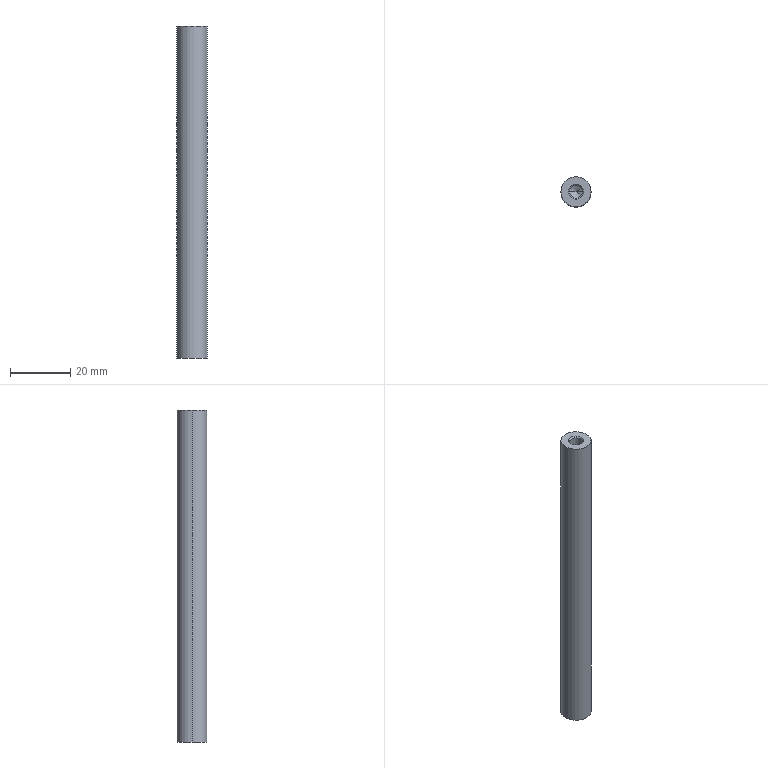Part | SolidWorks | features 3DProfileFeature 1, Extrusion 1, HoleWzd 1, MirrorPattern 1 | 1 solid | 16 faces | box 10 x 10 x 110 mm | volume 8282 mm3 | cone 8 | cylinder 6 | plane 2 | commonest cylinder face diameters 4.2 x4 10 x2
STEP:
#1=CARTESIAN_POINT('',(2.1,0.,-54.575));
#2=VERTEX_POINT('',#1);
#3=CARTESIAN_POINT('',(-2.1,0.,-54.575));
#4=VERTEX_POINT('',#3);
#5=CARTESIAN_POINT('',(0.,0.,-54.575));
#6=DIRECTION('',(0.,0.,-1.));
#7=DIRECTION('',(-1.,0.,0.));
#8=AXIS2_PLACEMENT_3D('',#5,#6,#7);
#9=CIRCLE('',#8,2.1);
#10=EDGE_CURVE('',#2,#4,#9,.T.);
#11=ORIENTED_EDGE('',*,*,#10,.F.);
#12=CARTESIAN_POINT('',(2.525,0.,-55.));
#13=VERTEX_POINT('',#12);
#14=CARTESIAN_POINT('',(2.525,0.,-55.));
#15=DIRECTION('',(0.7071,0.,-0.7071));
#16=VECTOR('',#15,1000.);
#17=LINE('',#14,#16);
#18=EDGE_CURVE('',#2,#13,#17,.T.);
#19=ORIENTED_EDGE('',*,*,#18,.T.);
#20=CARTESIAN_POINT('',(-2.525,0.,-55.));
#21=VERTEX_POINT('',#20);
#22=CARTESIAN_POINT('',(0.,0.,-55.));
#23=DIRECTION('',(0.,0.,-1.));
#24=DIRECTION('',(-1.,0.,0.));
#25=AXIS2_PLACEMENT_3D('',#22,#23,#24);
#26=CIRCLE('',#25,2.525);
#27=EDGE_CURVE('',#13,#21,#26,.T.);
#28=ORIENTED_EDGE('',*,*,#27,.T.);
#29=CARTESIAN_POINT('',(-2.525,0.,-55.));
#30=DIRECTION('',(-0.7071,0.,-0.7071));
#31=VECTOR('',#30,1000.);
#32=LINE('',#29,#31);
#33=EDGE_CURVE('',#4,#21,#32,.T.);
#34=ORIENTED_EDGE('',*,*,#33,.F.);
#35=EDGE_LOOP('',(#11,#19,#28,#34));
#36=FACE_OUTER_BOUND('',#35,.T.);
#37=CARTESIAN_POINT('',(0.,0.,-55.));
#38=DIRECTION('',(0.,0.,-1.));
#39=DIRECTION('',(-1.,0.,0.));
#40=AXIS2_PLACEMENT_3D('',#37,#38,#39);
#41=CONICAL_SURFACE('',#40,2.525,0.7854);
#42=ADVANCED_FACE('',(#36),#41,.F.);
#43=CARTESIAN_POINT('',(2.1,0.,-42.6));
#44=VERTEX_POINT('',#43);
#45=CARTESIAN_POINT('',(-2.1,0.,-42.6));
#46=VERTEX_POINT('',#45);
#47=CARTESIAN_POINT('',(0.,0.,-42.6));
#48=DIRECTION('',(0.,0.,-1.));
#49=DIRECTION('',(-1.,0.,0.));
#50=AXIS2_PLACEMENT_3D('',#47,#48,#49);
#51=CIRCLE('',#50,2.1);
#52=EDGE_CURVE('',#44,#46,#51,.T.);
#53=ORIENTED_EDGE('',*,*,#52,.F.);
#54=CARTESIAN_POINT('',(2.1,0.,-55.));
#55=DIRECTION('',(0.,0.,-1.));
#56=VECTOR('',#55,1000.);
#57=LINE('',#54,#56);
#58=EDGE_CURVE('',#44,#2,#57,.T.);
#59=ORIENTED_EDGE('',*,*,#58,.T.);
#60=ORIENTED_EDGE('',*,*,#10,.T.);
#61=CARTESIAN_POINT('',(-2.1,0.,-55.));
#62=DIRECTION('',(0.,0.,-1.));
#63=VECTOR('',#62,1000.);
#64=LINE('',#61,#63);
#65=EDGE_CURVE('',#46,#4,#64,.T.);
#66=ORIENTED_EDGE('',*,*,#65,.F.);
#67=EDGE_LOOP('',(#53,#59,#60,#66));
#68=FACE_OUTER_BOUND('',#67,.T.);
#69=CARTESIAN_POINT('',(0.,0.,-55.));
#70=DIRECTION('',(0.,0.,-1.));
#71=DIRECTION('',(-1.,0.,0.));
#72=AXIS2_PLACEMENT_3D('',#69,#70,#71);
#73=CYLINDRICAL_SURFACE('',#72,2.1);
#74=ADVANCED_FACE('',(#68),#73,.F.);
#75=CARTESIAN_POINT('',(0.,0.,-41.338));
#76=VERTEX_POINT('',#75);
#77=CARTESIAN_POINT('',(-2.1,0.,-42.6));
#78=DIRECTION('',(-0.8572,0.,-0.515));
#79=VECTOR('',#78,1000.);
#80=LINE('',#77,#79);
#81=EDGE_CURVE('',#76,#46,#80,.T.);
#82=ORIENTED_EDGE('',*,*,#81,.F.);
#83=CARTESIAN_POINT('',(2.1,0.,-42.6));
#84=DIRECTION('',(0.8572,0.,-0.515));
#85=VECTOR('',#84,1000.);
#86=LINE('',#83,#85);
#87=EDGE_CURVE('',#76,#44,#86,.T.);
#88=ORIENTED_EDGE('',*,*,#87,.T.);
#89=ORIENTED_EDGE('',*,*,#52,.T.);
#90=EDGE_LOOP('',(#82,#88,#89));
#91=FACE_OUTER_BOUND('',#90,.T.);
#92=CARTESIAN_POINT('',(0.,0.,-42.6));
#93=DIRECTION('',(0.,0.,-1.));
#94=DIRECTION('',(-1.,0.,0.));
#95=AXIS2_PLACEMENT_3D('',#92,#93,#94);
#96=CONICAL_SURFACE('',#95,2.1,1.03);
#97=ADVANCED_FACE('',(#91),#96,.F.);
#98=CARTESIAN_POINT('',(-2.1,0.,54.575));
#99=VERTEX_POINT('',#98);
#100=CARTESIAN_POINT('',(2.1,0.,54.575));
#101=VERTEX_POINT('',#100);
#102=CARTESIAN_POINT('',(0.,0.,54.575));
#103=DIRECTION('',(0.,0.,1.));
#104=DIRECTION('',(1.,0.,0.));
#105=AXIS2_PLACEMENT_3D('',#102,#103,#104);
#106=CIRCLE('',#105,2.1);
#107=EDGE_CURVE('',#99,#101,#106,.T.);
#108=ORIENTED_EDGE('',*,*,#107,.F.);
#109=CARTESIAN_POINT('',(-2.525,0.,55.));
#110=VERTEX_POINT('',#109);
#111=CARTESIAN_POINT('',(-2.525,0.,55.));
#112=DIRECTION('',(-0.7071,0.,0.7071));
#113=VECTOR('',#112,1000.);
#114=LINE('',#111,#113);
#115=EDGE_CURVE('',#99,#110,#114,.T.);
#116=ORIENTED_EDGE('',*,*,#115,.T.);
#117=CARTESIAN_POINT('',(2.525,0.,55.));
#118=VERTEX_POINT('',#117);
#119=CARTESIAN_POINT('',(0.,0.,55.));
#120=DIRECTION('',(0.,0.,1.));
#121=DIRECTION('',(1.,0.,0.));
#122=AXIS2_PLACEMENT_3D('',#119,#120,#121);
#123=CIRCLE('',#122,2.525);
#124=EDGE_CURVE('',#110,#118,#123,.T.);
#125=ORIENTED_EDGE('',*,*,#124,.T.);
#126=CARTESIAN_POINT('',(2.525,0.,55.));
#127=DIRECTION('',(0.7071,0.,0.7071));
#128=VECTOR('',#127,1000.);
#129=LINE('',#126,#128);
#130=EDGE_CURVE('',#101,#118,#129,.T.);
#131=ORIENTED_EDGE('',*,*,#130,.F.);
#132=EDGE_LOOP('',(#108,#116,#125,#131));
#133=FACE_OUTER_BOUND('',#132,.T.);
#134=CARTESIAN_POINT('',(0.,0.,55.));
#135=DIRECTION('',(0.,0.,1.));
#136=DIRECTION('',(1.,0.,0.));
#137=AXIS2_PLACEMENT_3D('',#134,#135,#136);
#138=CONICAL_SURFACE('',#137,2.525,0.7854);
#139=ADVANCED_FACE('',(#133),#138,.F.);
#140=CARTESIAN_POINT('',(-2.1,0.,42.6));
#141=VERTEX_POINT('',#140);
#142=CARTESIAN_POINT('',(2.1,0.,42.6));
#143=VERTEX_POINT('',#142);
#144=CARTESIAN_POINT('',(0.,0.,42.6));
#145=DIRECTION('',(0.,0.,1.));
#146=DIRECTION('',(1.,0.,0.));
#147=AXIS2_PLACEMENT_3D('',#144,#145,#146);
#148=CIRCLE('',#147,2.1);
#149=EDGE_CURVE('',#141,#143,#148,.T.);
#150=ORIENTED_EDGE('',*,*,#149,.F.);
#151=CARTESIAN_POINT('',(-2.1,0.,55.));
#152=DIRECTION('',(0.,0.,1.));
#153=VECTOR('',#152,1000.);
#154=LINE('',#151,#153);
#155=EDGE_CURVE('',#141,#99,#154,.T.);
#156=ORIENTED_EDGE('',*,*,#155,.T.);
#157=ORIENTED_EDGE('',*,*,#107,.T.);
#158=CARTESIAN_POINT('',(2.1,0.,55.));
#159=DIRECTION('',(0.,0.,1.));
#160=VECTOR('',#159,1000.);
#161=LINE('',#158,#160);
#162=EDGE_CURVE('',#143,#101,#161,.T.);
#163=ORIENTED_EDGE('',*,*,#162,.F.);
#164=EDGE_LOOP('',(#150,#156,#157,#163));
#165=FACE_OUTER_BOUND('',#164,.T.);
#166=CARTESIAN_POINT('',(0.,0.,55.));
#167=DIRECTION('',(0.,0.,1.));
#168=DIRECTION('',(1.,0.,0.));
#169=AXIS2_PLACEMENT_3D('',#166,#167,#168);
#170=CYLINDRICAL_SURFACE('',#169,2.1);
#171=ADVANCED_FACE('',(#165),#170,.F.);
#172=CARTESIAN_POINT('',(0.,0.,41.338));
#173=VERTEX_POINT('',#172);
#174=CARTESIAN_POINT('',(2.1,0.,42.6));
#175=DIRECTION('',(0.8572,0.,0.515));
#176=VECTOR('',#175,1000.);
#177=LINE('',#174,#176);
#178=EDGE_CURVE('',#173,#143,#177,.T.);
#179=ORIENTED_EDGE('',*,*,#178,.F.);
#180=CARTESIAN_POINT('',(-2.1,0.,42.6));
#181=DIRECTION('',(-0.8572,0.,0.515));
#182=VECTOR('',#181,1000.);
#183=LINE('',#180,#182);
#184=EDGE_CURVE('',#173,#141,#183,.T.);
#185=ORIENTED_EDGE('',*,*,#184,.T.);
#186=ORIENTED_EDGE('',*,*,#149,.T.);
#187=EDGE_LOOP('',(#179,#185,#186));
#188=FACE_OUTER_BOUND('',#187,.T.);
#189=CARTESIAN_POINT('',(0.,0.,42.6));
#190=DIRECTION('',(0.,0.,1.));
#191=DIRECTION('',(1.,0.,0.));
#192=AXIS2_PLACEMENT_3D('',#189,#190,#191);
#193=CONICAL_SURFACE('',#192,2.1,1.03);
#194=ADVANCED_FACE('',(#188),#193,.F.);
#195=CARTESIAN_POINT('',(5.,0.,55.));
#196=VERTEX_POINT('',#195);
#197=CARTESIAN_POINT('',(-5.,0.,55.));
#198=VERTEX_POINT('',#197);
#199=CARTESIAN_POINT('',(0.,0.,55.));
#200=DIRECTION('',(0.,0.,1.));
#201=DIRECTION('',(1.,0.,0.));
#202=AXIS2_PLACEMENT_3D('',#199,#200,#201);
#203=CIRCLE('',#202,5.);
#204=EDGE_CURVE('',#196,#198,#203,.T.);
#205=ORIENTED_EDGE('',*,*,#204,.F.);
#206=CARTESIAN_POINT('',(5.,0.,-55.));
#207=VERTEX_POINT('',#206);
#208=CARTESIAN_POINT('',(5.,0.,55.));
#209=DIRECTION('',(0.,0.,-1.));
#210=VECTOR('',#209,1000.);
#211=LINE('',#208,#210);
#212=EDGE_CURVE('',#196,#207,#211,.T.);
#213=ORIENTED_EDGE('',*,*,#212,.T.);
#214=CARTESIAN_POINT('',(-5.,0.,-55.));
#215=VERTEX_POINT('',#214);
#216=CARTESIAN_POINT('',(0.,0.,-55.));
#217=DIRECTION('',(0.,0.,1.));
#218=DIRECTION('',(1.,0.,0.));
#219=AXIS2_PLACEMENT_3D('',#216,#217,#218);
#220=CIRCLE('',#219,5.);
#221=EDGE_CURVE('',#207,#215,#220,.T.);
#222=ORIENTED_EDGE('',*,*,#221,.T.);
#223=CARTESIAN_POINT('',(-5.,0.,55.));
#224=DIRECTION('',(0.,0.,-1.));
#225=VECTOR('',#224,1000.);
#226=LINE('',#223,#225);
#227=EDGE_CURVE('',#198,#215,#226,.T.);
#228=ORIENTED_EDGE('',*,*,#227,.F.);
#229=EDGE_LOOP('',(#205,#213,#222,#228));
#230=FACE_OUTER_BOUND('',#229,.T.);
#231=CARTESIAN_POINT('',(0.,0.,55.));
#232=DIRECTION('',(0.,0.,-1.));
#233=DIRECTION('',(-1.,0.,0.));
#234=AXIS2_PLACEMENT_3D('',#231,#232,#233);
#235=CYLINDRICAL_SURFACE('',#234,5.);
#236=ADVANCED_FACE('',(#230),#235,.T.);
#237=ORIENTED_EDGE('',*,*,#212,.F.);
#238=CARTESIAN_POINT('',(0.,0.,55.));
#239=DIRECTION('',(0.,0.,1.));
#240=DIRECTION('',(1.,0.,0.));
#241=AXIS2_PLACEMENT_3D('',#238,#239,#240);
#242=CIRCLE('',#241,5.);
#243=EDGE_CURVE('',#198,#196,#242,.T.);
#244=ORIENTED_EDGE('',*,*,#243,.F.);
#245=ORIENTED_EDGE('',*,*,#227,.T.);
#246=CARTESIAN_POINT('',(0.,0.,-55.));
#247=DIRECTION('',(0.,0.,1.));
#248=DIRECTION('',(1.,0.,0.));
#249=AXIS2_PLACEMENT_3D('',#246,#247,#248);
#250=CIRCLE('',#249,5.);
#251=EDGE_CURVE('',#215,#207,#250,.T.);
#252=ORIENTED_EDGE('',*,*,#251,.T.);
#253=EDGE_LOOP('',(#237,#244,#245,#252));
#254=FACE_OUTER_BOUND('',#253,.T.);
#255=CARTESIAN_POINT('',(0.,0.,55.));
#256=DIRECTION('',(0.,0.,-1.));
#257=DIRECTION('',(-1.,0.,0.));
#258=AXIS2_PLACEMENT_3D('',#255,#256,#257);
#259=CYLINDRICAL_SURFACE('',#258,5.);
#260=ADVANCED_FACE('',(#254),#259,.T.);
#261=CARTESIAN_POINT('',(0.,0.,55.));
#262=DIRECTION('',(0.,0.,1.));
#263=DIRECTION('',(1.,0.,0.));
#264=AXIS2_PLACEMENT_3D('',#261,#262,#263);
#265=CIRCLE('',#264,2.525);
#266=EDGE_CURVE('',#118,#110,#265,.T.);
#267=ORIENTED_EDGE('',*,*,#266,.F.);
#268=ORIENTED_EDGE('',*,*,#124,.F.);
#269=EDGE_LOOP('',(#267,#268));
#270=FACE_BOUND('',#269,.T.);
#271=ORIENTED_EDGE('',*,*,#243,.T.);
#272=ORIENTED_EDGE('',*,*,#204,.T.);
#273=EDGE_LOOP('',(#271,#272));
#274=FACE_OUTER_BOUND('',#273,.T.);
#275=CARTESIAN_POINT('',(0.,0.,55.));
#276=DIRECTION('',(0.,0.,1.));
#277=DIRECTION('',(1.,0.,0.));
#278=AXIS2_PLACEMENT_3D('',#275,#276,#277);
#279=PLANE('',#278);
#280=ADVANCED_FACE('',(#270,#274),#279,.T.);
#281=CARTESIAN_POINT('',(0.,0.,-55.));
#282=DIRECTION('',(0.,0.,-1.));
#283=DIRECTION('',(-1.,0.,0.));
#284=AXIS2_PLACEMENT_3D('',#281,#282,#283);
#285=CIRCLE('',#284,2.525);
#286=EDGE_CURVE('',#21,#13,#285,.T.);
#287=ORIENTED_EDGE('',*,*,#286,.F.);
#288=ORIENTED_EDGE('',*,*,#27,.F.);
#289=EDGE_LOOP('',(#287,#288));
#290=FACE_BOUND('',#289,.T.);
#291=ORIENTED_EDGE('',*,*,#251,.F.);
#292=ORIENTED_EDGE('',*,*,#221,.F.);
#293=EDGE_LOOP('',(#291,#292));
#294=FACE_OUTER_BOUND('',#293,.T.);
#295=CARTESIAN_POINT('',(0.,0.,-55.));
#296=DIRECTION('',(0.,0.,1.));
#297=DIRECTION('',(1.,0.,0.));
#298=AXIS2_PLACEMENT_3D('',#295,#296,#297);
#299=PLANE('',#298);
#300=ADVANCED_FACE('',(#290,#294),#299,.F.);
#301=ORIENTED_EDGE('',*,*,#184,.F.);
#302=ORIENTED_EDGE('',*,*,#178,.T.);
#303=CARTESIAN_POINT('',(0.,0.,42.6));
#304=DIRECTION('',(0.,0.,1.));
#305=DIRECTION('',(1.,0.,0.));
#306=AXIS2_PLACEMENT_3D('',#303,#304,#305);
#307=CIRCLE('',#306,2.1);
#308=EDGE_CURVE('',#143,#141,#307,.T.);
#309=ORIENTED_EDGE('',*,*,#308,.T.);
#310=EDGE_LOOP('',(#301,#302,#309));
#311=FACE_OUTER_BOUND('',#310,.T.);
#312=CARTESIAN_POINT('',(0.,0.,42.6));
#313=DIRECTION('',(0.,0.,1.));
#314=DIRECTION('',(1.,0.,0.));
#315=AXIS2_PLACEMENT_3D('',#312,#313,#314);
#316=CONICAL_SURFACE('',#315,2.1,1.03);
#317=ADVANCED_FACE('',(#311),#316,.F.);
#318=ORIENTED_EDGE('',*,*,#155,.F.);
#319=ORIENTED_EDGE('',*,*,#308,.F.);
#320=ORIENTED_EDGE('',*,*,#162,.T.);
#321=CARTESIAN_POINT('',(0.,0.,54.575));
#322=DIRECTION('',(0.,0.,1.));
#323=DIRECTION('',(1.,0.,0.));
#324=AXIS2_PLACEMENT_3D('',#321,#322,#323);
#325=CIRCLE('',#324,2.1);
#326=EDGE_CURVE('',#101,#99,#325,.T.);
#327=ORIENTED_EDGE('',*,*,#326,.T.);
#328=EDGE_LOOP('',(#318,#319,#320,#327));
#329=FACE_OUTER_BOUND('',#328,.T.);
#330=CARTESIAN_POINT('',(0.,0.,55.));
#331=DIRECTION('',(0.,0.,1.));
#332=DIRECTION('',(1.,0.,0.));
#333=AXIS2_PLACEMENT_3D('',#330,#331,#332);
#334=CYLINDRICAL_SURFACE('',#333,2.1);
#335=ADVANCED_FACE('',(#329),#334,.F.);
#336=ORIENTED_EDGE('',*,*,#115,.F.);
#337=ORIENTED_EDGE('',*,*,#326,.F.);
#338=ORIENTED_EDGE('',*,*,#130,.T.);
#339=ORIENTED_EDGE('',*,*,#266,.T.);
#340=EDGE_LOOP('',(#336,#337,#338,#339));
#341=FACE_OUTER_BOUND('',#340,.T.);
#342=CARTESIAN_POINT('',(0.,0.,55.));
#343=DIRECTION('',(0.,0.,1.));
#344=DIRECTION('',(1.,0.,0.));
#345=AXIS2_PLACEMENT_3D('',#342,#343,#344);
#346=CONICAL_SURFACE('',#345,2.525,0.7854);
#347=ADVANCED_FACE('',(#341),#346,.F.);
#348=ORIENTED_EDGE('',*,*,#87,.F.);
#349=ORIENTED_EDGE('',*,*,#81,.T.);
#350=CARTESIAN_POINT('',(0.,0.,-42.6));
#351=DIRECTION('',(0.,0.,-1.));
#352=DIRECTION('',(-1.,0.,0.));
#353=AXIS2_PLACEMENT_3D('',#350,#351,#352);
#354=CIRCLE('',#353,2.1);
#355=EDGE_CURVE('',#46,#44,#354,.T.);
#356=ORIENTED_EDGE('',*,*,#355,.T.);
#357=EDGE_LOOP('',(#348,#349,#356));
#358=FACE_OUTER_BOUND('',#357,.T.);
#359=CARTESIAN_POINT('',(0.,0.,-42.6));
#360=DIRECTION('',(0.,0.,-1.));
#361=DIRECTION('',(-1.,0.,0.));
#362=AXIS2_PLACEMENT_3D('',#359,#360,#361);
#363=CONICAL_SURFACE('',#362,2.1,1.03);
#364=ADVANCED_FACE('',(#358),#363,.F.);
#365=ORIENTED_EDGE('',*,*,#58,.F.);
#366=ORIENTED_EDGE('',*,*,#355,.F.);
#367=ORIENTED_EDGE('',*,*,#65,.T.);
#368=CARTESIAN_POINT('',(0.,0.,-54.575));
#369=DIRECTION('',(0.,0.,-1.));
#370=DIRECTION('',(-1.,0.,0.));
#371=AXIS2_PLACEMENT_3D('',#368,#369,#370);
#372=CIRCLE('',#371,2.1);
#373=EDGE_CURVE('',#4,#2,#372,.T.);
#374=ORIENTED_EDGE('',*,*,#373,.T.);
#375=EDGE_LOOP('',(#365,#366,#367,#374));
#376=FACE_OUTER_BOUND('',#375,.T.);
#377=CARTESIAN_POINT('',(0.,0.,-55.));
#378=DIRECTION('',(0.,0.,-1.));
#379=DIRECTION('',(-1.,0.,0.));
#380=AXIS2_PLACEMENT_3D('',#377,#378,#379);
#381=CYLINDRICAL_SURFACE('',#380,2.1);
#382=ADVANCED_FACE('',(#376),#381,.F.);
#383=ORIENTED_EDGE('',*,*,#18,.F.);
#384=ORIENTED_EDGE('',*,*,#373,.F.);
#385=ORIENTED_EDGE('',*,*,#33,.T.);
#386=ORIENTED_EDGE('',*,*,#286,.T.);
#387=EDGE_LOOP('',(#383,#384,#385,#386));
#388=FACE_OUTER_BOUND('',#387,.T.);
#389=CARTESIAN_POINT('',(0.,0.,-55.));
#390=DIRECTION('',(0.,0.,-1.));
#391=DIRECTION('',(-1.,0.,0.));
#392=AXIS2_PLACEMENT_3D('',#389,#390,#391);
#393=CONICAL_SURFACE('',#392,2.525,0.7854);
#394=ADVANCED_FACE('',(#388),#393,.F.);
#395=CLOSED_SHELL('',(#42,#74,#97,#139,#171,#194,#236,#260,#280,#300,#317,#335,#347,#364,#382,#394));
#396=MANIFOLD_SOLID_BREP('',#395);
#397=CARTESIAN_POINT('',(0.,0.,0.));
#398=DIRECTION('',(0.,0.,1.));
#399=DIRECTION('',(1.,0.,0.));
#400=AXIS2_PLACEMENT_3D('',#397,#398,#399);
#401=(LENGTH_UNIT()NAMED_UNIT(*)SI_UNIT(.MILLI.,.METRE.));
#402=UNCERTAINTY_MEASURE_WITH_UNIT(LENGTH_MEASURE(0.00001),#401,'','');
#403=(NAMED_UNIT(*)PLANE_ANGLE_UNIT()SI_UNIT($,.RADIAN.));
#404=(NAMED_UNIT(*)SI_UNIT($,.STERADIAN.)SOLID_ANGLE_UNIT());
#405=(GEOMETRIC_REPRESENTATION_CONTEXT(3)GLOBAL_UNCERTAINTY_ASSIGNED_CONTEXT((#402))GLOBAL_UNIT_ASSIGNED_CONTEXT((#401,#403,#404))REPRESENTATION_CONTEXT('',''));
#406=ADVANCED_BREP_SHAPE_REPRESENTATION('',(#396,#400),#405);